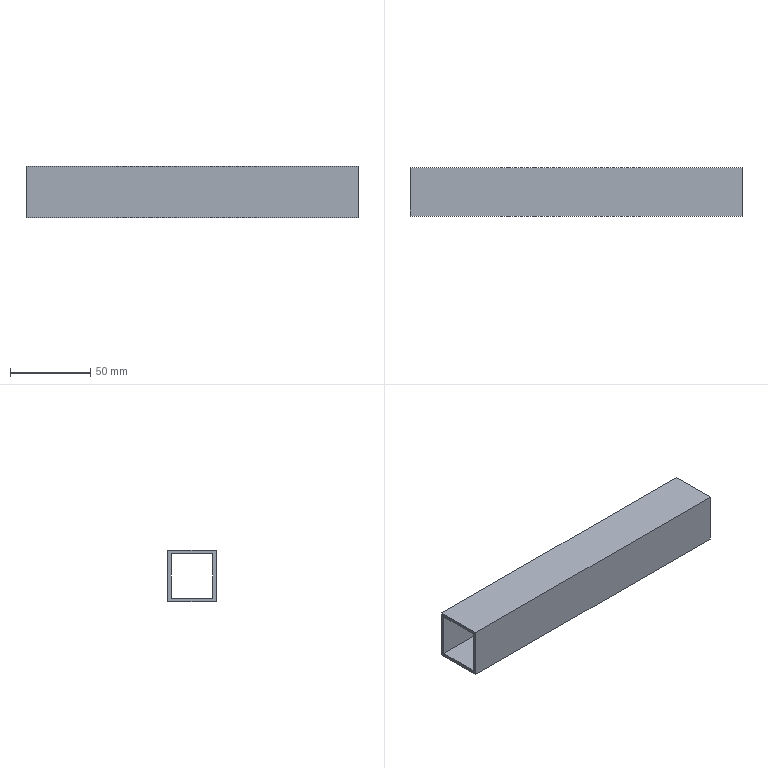Part | NX | features solid 2 | 1 solid | 10 faces | box 207 x 30 x 32 mm | volume 48024 mm3 | plane 10
STEP:
#1=CARTESIAN_POINT('',(-43.,575.,-63.));
#2=VERTEX_POINT('',#1);
#3=CARTESIAN_POINT('',(-43.,545.,-63.));
#4=VERTEX_POINT('',#3);
#5=CARTESIAN_POINT('',(-43.,545.,-63.));
#6=DIRECTION('',(0.,1.,0.));
#7=VECTOR('',#6,1000.);
#8=LINE('',#5,#7);
#9=EDGE_CURVE('',#2,#4,#8,.F.);
#10=ORIENTED_EDGE('',*,*,#9,.T.);
#11=CARTESIAN_POINT('',(-43.,545.,-95.));
#12=VERTEX_POINT('',#11);
#13=CARTESIAN_POINT('',(-43.,545.,-63.));
#14=DIRECTION('',(0.,0.,1.));
#15=VECTOR('',#14,1000.);
#16=LINE('',#13,#15);
#17=EDGE_CURVE('',#4,#12,#16,.F.);
#18=ORIENTED_EDGE('',*,*,#17,.T.);
#19=CARTESIAN_POINT('',(-43.,575.,-95.));
#20=VERTEX_POINT('',#19);
#21=CARTESIAN_POINT('',(-43.,545.,-95.));
#22=DIRECTION('',(0.,-1.,0.));
#23=VECTOR('',#22,1000.);
#24=LINE('',#21,#23);
#25=EDGE_CURVE('',#20,#12,#24,.T.);
#26=ORIENTED_EDGE('',*,*,#25,.F.);
#27=CARTESIAN_POINT('',(-43.,575.,-63.));
#28=DIRECTION('',(0.,0.,1.));
#29=VECTOR('',#28,1000.);
#30=LINE('',#27,#29);
#31=EDGE_CURVE('',#2,#20,#30,.F.);
#32=ORIENTED_EDGE('',*,*,#31,.F.);
#33=EDGE_LOOP('',(#10,#18,#26,#32));
#34=FACE_BOUND('',#33,.T.);
#35=CARTESIAN_POINT('',(-43.,573.,-65.));
#36=VERTEX_POINT('',#35);
#37=CARTESIAN_POINT('',(-43.,547.,-65.));
#38=VERTEX_POINT('',#37);
#39=CARTESIAN_POINT('',(-43.,545.,-65.));
#40=DIRECTION('',(0.,1.,0.));
#41=VECTOR('',#40,1000.);
#42=LINE('',#39,#41);
#43=EDGE_CURVE('',#36,#38,#42,.F.);
#44=ORIENTED_EDGE('',*,*,#43,.F.);
#45=CARTESIAN_POINT('',(-43.,573.,-93.));
#46=VERTEX_POINT('',#45);
#47=CARTESIAN_POINT('',(-43.,573.,-63.));
#48=DIRECTION('',(0.,0.,1.));
#49=VECTOR('',#48,1000.);
#50=LINE('',#47,#49);
#51=EDGE_CURVE('',#36,#46,#50,.F.);
#52=ORIENTED_EDGE('',*,*,#51,.T.);
#53=CARTESIAN_POINT('',(-43.,547.,-93.));
#54=VERTEX_POINT('',#53);
#55=CARTESIAN_POINT('',(-43.,545.,-93.));
#56=DIRECTION('',(0.,-1.,0.));
#57=VECTOR('',#56,1000.);
#58=LINE('',#55,#57);
#59=EDGE_CURVE('',#46,#54,#58,.T.);
#60=ORIENTED_EDGE('',*,*,#59,.T.);
#61=CARTESIAN_POINT('',(-43.,547.,-63.));
#62=DIRECTION('',(0.,0.,1.));
#63=VECTOR('',#62,1000.);
#64=LINE('',#61,#63);
#65=EDGE_CURVE('',#38,#54,#64,.F.);
#66=ORIENTED_EDGE('',*,*,#65,.F.);
#67=EDGE_LOOP('',(#44,#52,#60,#66));
#68=FACE_BOUND('',#67,.T.);
#69=CARTESIAN_POINT('',(-43.,545.,-63.));
#70=DIRECTION('',(1.,0.,0.));
#71=DIRECTION('',(0.,0.,-1.));
#72=AXIS2_PLACEMENT_3D('',#69,#70,#71);
#73=PLANE('',#72);
#74=ADVANCED_FACE('',(#34,#68),#73,.T.);
#75=CARTESIAN_POINT('',(-250.,575.,-95.));
#76=VERTEX_POINT('',#75);
#77=CARTESIAN_POINT('',(-250.,545.,-95.));
#78=VERTEX_POINT('',#77);
#79=CARTESIAN_POINT('',(-250.,378.,-95.));
#80=DIRECTION('',(0.,1.,0.));
#81=VECTOR('',#80,1000.);
#82=LINE('',#79,#81);
#83=EDGE_CURVE('',#76,#78,#82,.F.);
#84=ORIENTED_EDGE('',*,*,#83,.T.);
#85=CARTESIAN_POINT('',(-250.,545.,-63.));
#86=VERTEX_POINT('',#85);
#87=CARTESIAN_POINT('',(-250.,545.,-63.));
#88=DIRECTION('',(0.,0.,-1.));
#89=VECTOR('',#88,1000.);
#90=LINE('',#87,#89);
#91=EDGE_CURVE('',#86,#78,#90,.T.);
#92=ORIENTED_EDGE('',*,*,#91,.F.);
#93=CARTESIAN_POINT('',(-250.,575.,-63.));
#94=VERTEX_POINT('',#93);
#95=CARTESIAN_POINT('',(-250.,545.,-63.));
#96=DIRECTION('',(0.,-1.,0.));
#97=VECTOR('',#96,1000.);
#98=LINE('',#95,#97);
#99=EDGE_CURVE('',#94,#86,#98,.T.);
#100=ORIENTED_EDGE('',*,*,#99,.F.);
#101=CARTESIAN_POINT('',(-250.,575.,-63.));
#102=DIRECTION('',(0.,0.,-1.));
#103=VECTOR('',#102,1000.);
#104=LINE('',#101,#103);
#105=EDGE_CURVE('',#94,#76,#104,.T.);
#106=ORIENTED_EDGE('',*,*,#105,.T.);
#107=EDGE_LOOP('',(#84,#92,#100,#106));
#108=FACE_BOUND('',#107,.T.);
#109=CARTESIAN_POINT('',(-250.,573.,-93.));
#110=VERTEX_POINT('',#109);
#111=CARTESIAN_POINT('',(-250.,547.,-93.));
#112=VERTEX_POINT('',#111);
#113=CARTESIAN_POINT('',(-250.,378.,-93.));
#114=DIRECTION('',(0.,1.,0.));
#115=VECTOR('',#114,1000.);
#116=LINE('',#113,#115);
#117=EDGE_CURVE('',#110,#112,#116,.F.);
#118=ORIENTED_EDGE('',*,*,#117,.F.);
#119=CARTESIAN_POINT('',(-250.,573.,-65.));
#120=VERTEX_POINT('',#119);
#121=CARTESIAN_POINT('',(-250.,573.,-63.));
#122=DIRECTION('',(0.,0.,-1.));
#123=VECTOR('',#122,1000.);
#124=LINE('',#121,#123);
#125=EDGE_CURVE('',#120,#110,#124,.T.);
#126=ORIENTED_EDGE('',*,*,#125,.F.);
#127=CARTESIAN_POINT('',(-250.,547.,-65.));
#128=VERTEX_POINT('',#127);
#129=CARTESIAN_POINT('',(-250.,545.,-65.));
#130=DIRECTION('',(0.,-1.,0.));
#131=VECTOR('',#130,1000.);
#132=LINE('',#129,#131);
#133=EDGE_CURVE('',#120,#128,#132,.T.);
#134=ORIENTED_EDGE('',*,*,#133,.T.);
#135=CARTESIAN_POINT('',(-250.,547.,-63.));
#136=DIRECTION('',(0.,0.,-1.));
#137=VECTOR('',#136,1000.);
#138=LINE('',#135,#137);
#139=EDGE_CURVE('',#128,#112,#138,.T.);
#140=ORIENTED_EDGE('',*,*,#139,.T.);
#141=EDGE_LOOP('',(#118,#126,#134,#140));
#142=FACE_BOUND('',#141,.T.);
#143=CARTESIAN_POINT('',(-250.,378.,-63.));
#144=DIRECTION('',(1.,0.,0.));
#145=DIRECTION('',(0.,0.,1.));
#146=AXIS2_PLACEMENT_3D('',#143,#144,#145);
#147=PLANE('',#146);
#148=ADVANCED_FACE('',(#108,#142),#147,.F.);
#149=ORIENTED_EDGE('',*,*,#25,.T.);
#150=CARTESIAN_POINT('',(-53.,545.,-95.));
#151=DIRECTION('',(-1.,0.,0.));
#152=VECTOR('',#151,1000.);
#153=LINE('',#150,#152);
#154=EDGE_CURVE('',#12,#78,#153,.T.);
#155=ORIENTED_EDGE('',*,*,#154,.T.);
#156=ORIENTED_EDGE('',*,*,#83,.F.);
#157=CARTESIAN_POINT('',(-53.,575.,-95.));
#158=DIRECTION('',(1.,0.,0.));
#159=VECTOR('',#158,1000.);
#160=LINE('',#157,#159);
#161=EDGE_CURVE('',#20,#76,#160,.F.);
#162=ORIENTED_EDGE('',*,*,#161,.F.);
#163=EDGE_LOOP('',(#149,#155,#156,#162));
#164=FACE_BOUND('',#163,.T.);
#165=CARTESIAN_POINT('',(-53.,545.,-95.));
#166=DIRECTION('',(0.,0.,-1.));
#167=DIRECTION('',(-1.,0.,0.));
#168=AXIS2_PLACEMENT_3D('',#165,#166,#167);
#169=PLANE('',#168);
#170=ADVANCED_FACE('',(#164),#169,.T.);
#171=CARTESIAN_POINT('',(-53.,575.,-63.));
#172=DIRECTION('',(-1.,0.,0.));
#173=VECTOR('',#172,1000.);
#174=LINE('',#171,#173);
#175=EDGE_CURVE('',#2,#94,#174,.T.);
#176=ORIENTED_EDGE('',*,*,#175,.T.);
#177=ORIENTED_EDGE('',*,*,#99,.T.);
#178=CARTESIAN_POINT('',(-53.,545.,-63.));
#179=DIRECTION('',(-1.,0.,0.));
#180=VECTOR('',#179,1000.);
#181=LINE('',#178,#180);
#182=EDGE_CURVE('',#4,#86,#181,.T.);
#183=ORIENTED_EDGE('',*,*,#182,.F.);
#184=ORIENTED_EDGE('',*,*,#9,.F.);
#185=EDGE_LOOP('',(#176,#177,#183,#184));
#186=FACE_BOUND('',#185,.T.);
#187=CARTESIAN_POINT('',(-53.,545.,-63.));
#188=DIRECTION('',(0.,0.,-1.));
#189=DIRECTION('',(-1.,0.,0.));
#190=AXIS2_PLACEMENT_3D('',#187,#188,#189);
#191=PLANE('',#190);
#192=ADVANCED_FACE('',(#186),#191,.F.);
#193=ORIENTED_EDGE('',*,*,#91,.T.);
#194=ORIENTED_EDGE('',*,*,#154,.F.);
#195=ORIENTED_EDGE('',*,*,#17,.F.);
#196=ORIENTED_EDGE('',*,*,#182,.T.);
#197=EDGE_LOOP('',(#193,#194,#195,#196));
#198=FACE_BOUND('',#197,.T.);
#199=CARTESIAN_POINT('',(-53.,545.,-63.));
#200=DIRECTION('',(0.,1.,0.));
#201=DIRECTION('',(0.,0.,1.));
#202=AXIS2_PLACEMENT_3D('',#199,#200,#201);
#203=PLANE('',#202);
#204=ADVANCED_FACE('',(#198),#203,.F.);
#205=ORIENTED_EDGE('',*,*,#105,.F.);
#206=ORIENTED_EDGE('',*,*,#175,.F.);
#207=ORIENTED_EDGE('',*,*,#31,.T.);
#208=ORIENTED_EDGE('',*,*,#161,.T.);
#209=EDGE_LOOP('',(#205,#206,#207,#208));
#210=FACE_BOUND('',#209,.T.);
#211=CARTESIAN_POINT('',(-53.,575.,-63.));
#212=DIRECTION('',(0.,1.,0.));
#213=DIRECTION('',(0.,0.,1.));
#214=AXIS2_PLACEMENT_3D('',#211,#212,#213);
#215=PLANE('',#214);
#216=ADVANCED_FACE('',(#210),#215,.T.);
#217=CARTESIAN_POINT('',(-53.,547.,-93.));
#218=DIRECTION('',(1.,0.,0.));
#219=VECTOR('',#218,1000.);
#220=LINE('',#217,#219);
#221=EDGE_CURVE('',#54,#112,#220,.F.);
#222=ORIENTED_EDGE('',*,*,#221,.F.);
#223=ORIENTED_EDGE('',*,*,#59,.F.);
#224=CARTESIAN_POINT('',(-53.,573.,-93.));
#225=DIRECTION('',(1.,0.,0.));
#226=VECTOR('',#225,1000.);
#227=LINE('',#224,#226);
#228=EDGE_CURVE('',#46,#110,#227,.F.);
#229=ORIENTED_EDGE('',*,*,#228,.T.);
#230=ORIENTED_EDGE('',*,*,#117,.T.);
#231=EDGE_LOOP('',(#222,#223,#229,#230));
#232=FACE_BOUND('',#231,.T.);
#233=CARTESIAN_POINT('',(-53.,545.,-93.));
#234=DIRECTION('',(0.,0.,-1.));
#235=DIRECTION('',(-1.,0.,0.));
#236=AXIS2_PLACEMENT_3D('',#233,#234,#235);
#237=PLANE('',#236);
#238=ADVANCED_FACE('',(#232),#237,.F.);
#239=CARTESIAN_POINT('',(-53.,573.,-65.));
#240=DIRECTION('',(-1.,0.,0.));
#241=VECTOR('',#240,1000.);
#242=LINE('',#239,#241);
#243=EDGE_CURVE('',#36,#120,#242,.T.);
#244=ORIENTED_EDGE('',*,*,#243,.F.);
#245=ORIENTED_EDGE('',*,*,#43,.T.);
#246=CARTESIAN_POINT('',(-53.,547.,-65.));
#247=DIRECTION('',(-1.,0.,0.));
#248=VECTOR('',#247,1000.);
#249=LINE('',#246,#248);
#250=EDGE_CURVE('',#38,#128,#249,.T.);
#251=ORIENTED_EDGE('',*,*,#250,.T.);
#252=ORIENTED_EDGE('',*,*,#133,.F.);
#253=EDGE_LOOP('',(#244,#245,#251,#252));
#254=FACE_BOUND('',#253,.T.);
#255=CARTESIAN_POINT('',(-53.,545.,-65.));
#256=DIRECTION('',(0.,0.,-1.));
#257=DIRECTION('',(-1.,0.,0.));
#258=AXIS2_PLACEMENT_3D('',#255,#256,#257);
#259=PLANE('',#258);
#260=ADVANCED_FACE('',(#254),#259,.T.);
#261=ORIENTED_EDGE('',*,*,#139,.F.);
#262=ORIENTED_EDGE('',*,*,#250,.F.);
#263=ORIENTED_EDGE('',*,*,#65,.T.);
#264=ORIENTED_EDGE('',*,*,#221,.T.);
#265=EDGE_LOOP('',(#261,#262,#263,#264));
#266=FACE_BOUND('',#265,.T.);
#267=CARTESIAN_POINT('',(-53.,547.,-63.));
#268=DIRECTION('',(0.,1.,0.));
#269=DIRECTION('',(0.,0.,1.));
#270=AXIS2_PLACEMENT_3D('',#267,#268,#269);
#271=PLANE('',#270);
#272=ADVANCED_FACE('',(#266),#271,.T.);
#273=ORIENTED_EDGE('',*,*,#125,.T.);
#274=ORIENTED_EDGE('',*,*,#228,.F.);
#275=ORIENTED_EDGE('',*,*,#51,.F.);
#276=ORIENTED_EDGE('',*,*,#243,.T.);
#277=EDGE_LOOP('',(#273,#274,#275,#276));
#278=FACE_BOUND('',#277,.T.);
#279=CARTESIAN_POINT('',(-53.,573.,-63.));
#280=DIRECTION('',(0.,1.,0.));
#281=DIRECTION('',(0.,0.,1.));
#282=AXIS2_PLACEMENT_3D('',#279,#280,#281);
#283=PLANE('',#282);
#284=ADVANCED_FACE('',(#278),#283,.F.);
#285=CLOSED_SHELL('',(#74,#148,#170,#192,#204,#216,#238,#260,#272,#284));
#286=MANIFOLD_SOLID_BREP('',#285);
#287=(LENGTH_UNIT()NAMED_UNIT(*)SI_UNIT(.MILLI.,.METRE.));
#288=UNCERTAINTY_MEASURE_WITH_UNIT(LENGTH_MEASURE(0.00001),#287,'','');
#289=(NAMED_UNIT(*)PLANE_ANGLE_UNIT()SI_UNIT($,.RADIAN.));
#290=(NAMED_UNIT(*)SI_UNIT($,.STERADIAN.)SOLID_ANGLE_UNIT());
#291=(GEOMETRIC_REPRESENTATION_CONTEXT(3)GLOBAL_UNCERTAINTY_ASSIGNED_CONTEXT((#288))GLOBAL_UNIT_ASSIGNED_CONTEXT((#287,#289,#290))REPRESENTATION_CONTEXT('',''));
#292=ADVANCED_BREP_SHAPE_REPRESENTATION('',(#286),#291);